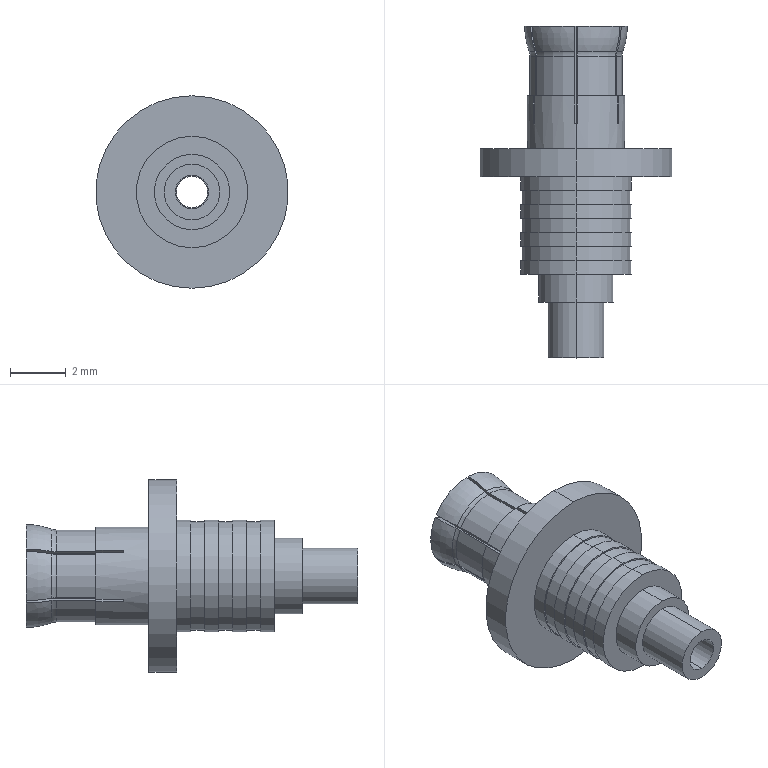Part | SolidWorks | features ICE 4, CirPattern 1, Revolution 1 | 1 solid | 99 faces | box 6.9 x 11.9 x 6.9 mm | volume 89.557 mm3 | plane 47 | cylinder 40 | torus 12 | commonest cylinder face diameters 4 x8 3.3 x6 3.9 x6 2.7 x5 2.9 x3 1.13 x2